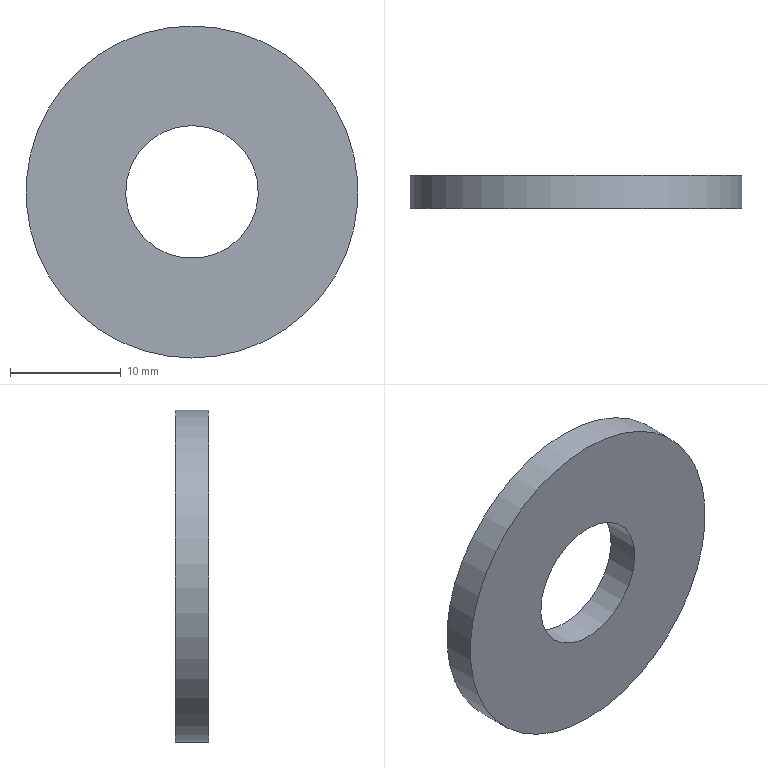Part | NX | features solid 2 | 1 solid | 4 faces | box 30 x 3 x 30 mm | volume 1781 mm3 | cylinder 2 | plane 2 | commonest cylinder face diameters 12 x1 30 x1
STEP:
#1=CARTESIAN_POINT('',(0.,618.,-111.));
#2=VERTEX_POINT('',#1);
#3=CARTESIAN_POINT('',(0.,618.,-117.));
#4=DIRECTION('',(0.,1.,0.));
#5=DIRECTION('',(0.,0.,1.));
#6=AXIS2_PLACEMENT_3D('',#3,#4,#5);
#7=CIRCLE('',#6,6.);
#8=EDGE_CURVE('',#2,#2,#7,.F.);
#9=ORIENTED_EDGE('',*,*,#8,.F.);
#10=EDGE_LOOP('',(#9));
#11=FACE_BOUND('',#10,.T.);
#12=CARTESIAN_POINT('',(0.,615.,-111.));
#13=VERTEX_POINT('',#12);
#14=CARTESIAN_POINT('',(0.,615.,-117.));
#15=DIRECTION('',(0.,1.,0.));
#16=DIRECTION('',(0.,0.,1.));
#17=AXIS2_PLACEMENT_3D('',#14,#15,#16);
#18=CIRCLE('',#17,6.);
#19=EDGE_CURVE('',#13,#13,#18,.F.);
#20=ORIENTED_EDGE('',*,*,#19,.T.);
#21=EDGE_LOOP('',(#20));
#22=FACE_BOUND('',#21,.T.);
#23=CARTESIAN_POINT('',(0.,615.,-117.));
#24=DIRECTION('',(0.,1.,0.));
#25=DIRECTION('',(0.,0.,1.));
#26=AXIS2_PLACEMENT_3D('',#23,#24,#25);
#27=CYLINDRICAL_SURFACE('',#26,6.);
#28=ADVANCED_FACE('',(#11,#22),#27,.F.);
#29=ORIENTED_EDGE('',*,*,#19,.F.);
#30=EDGE_LOOP('',(#29));
#31=FACE_BOUND('',#30,.T.);
#32=CARTESIAN_POINT('',(0.,615.,-102.));
#33=VERTEX_POINT('',#32);
#34=CARTESIAN_POINT('',(0.,615.,-117.));
#35=DIRECTION('',(0.,1.,0.));
#36=DIRECTION('',(0.,0.,1.));
#37=AXIS2_PLACEMENT_3D('',#34,#35,#36);
#38=CIRCLE('',#37,15.);
#39=EDGE_CURVE('',#33,#33,#38,.F.);
#40=ORIENTED_EDGE('',*,*,#39,.T.);
#41=EDGE_LOOP('',(#40));
#42=FACE_BOUND('',#41,.T.);
#43=CARTESIAN_POINT('',(0.,615.,-117.));
#44=DIRECTION('',(0.,1.,0.));
#45=DIRECTION('',(0.,0.,1.));
#46=AXIS2_PLACEMENT_3D('',#43,#44,#45);
#47=PLANE('',#46);
#48=ADVANCED_FACE('',(#31,#42),#47,.F.);
#49=ORIENTED_EDGE('',*,*,#8,.T.);
#50=EDGE_LOOP('',(#49));
#51=FACE_BOUND('',#50,.T.);
#52=CARTESIAN_POINT('',(0.,618.,-102.));
#53=VERTEX_POINT('',#52);
#54=CARTESIAN_POINT('',(0.,618.,-117.));
#55=DIRECTION('',(0.,1.,0.));
#56=DIRECTION('',(0.,0.,1.));
#57=AXIS2_PLACEMENT_3D('',#54,#55,#56);
#58=CIRCLE('',#57,15.);
#59=EDGE_CURVE('',#53,#53,#58,.F.);
#60=ORIENTED_EDGE('',*,*,#59,.F.);
#61=EDGE_LOOP('',(#60));
#62=FACE_BOUND('',#61,.T.);
#63=CARTESIAN_POINT('',(0.,618.,-117.));
#64=DIRECTION('',(0.,1.,0.));
#65=DIRECTION('',(0.,0.,1.));
#66=AXIS2_PLACEMENT_3D('',#63,#64,#65);
#67=PLANE('',#66);
#68=ADVANCED_FACE('',(#51,#62),#67,.T.);
#69=ORIENTED_EDGE('',*,*,#59,.T.);
#70=EDGE_LOOP('',(#69));
#71=FACE_BOUND('',#70,.T.);
#72=ORIENTED_EDGE('',*,*,#39,.F.);
#73=EDGE_LOOP('',(#72));
#74=FACE_BOUND('',#73,.T.);
#75=CARTESIAN_POINT('',(0.,615.,-117.));
#76=DIRECTION('',(0.,1.,0.));
#77=DIRECTION('',(0.,0.,1.));
#78=AXIS2_PLACEMENT_3D('',#75,#76,#77);
#79=CYLINDRICAL_SURFACE('',#78,15.);
#80=ADVANCED_FACE('',(#71,#74),#79,.T.);
#81=CLOSED_SHELL('',(#28,#48,#68,#80));
#82=MANIFOLD_SOLID_BREP('',#81);
#83=(LENGTH_UNIT()NAMED_UNIT(*)SI_UNIT(.MILLI.,.METRE.));
#84=UNCERTAINTY_MEASURE_WITH_UNIT(LENGTH_MEASURE(0.00001),#83,'','');
#85=(NAMED_UNIT(*)PLANE_ANGLE_UNIT()SI_UNIT($,.RADIAN.));
#86=(NAMED_UNIT(*)SI_UNIT($,.STERADIAN.)SOLID_ANGLE_UNIT());
#87=(GEOMETRIC_REPRESENTATION_CONTEXT(3)GLOBAL_UNCERTAINTY_ASSIGNED_CONTEXT((#84))GLOBAL_UNIT_ASSIGNED_CONTEXT((#83,#85,#86))REPRESENTATION_CONTEXT('',''));
#88=ADVANCED_BREP_SHAPE_REPRESENTATION('',(#82),#87);